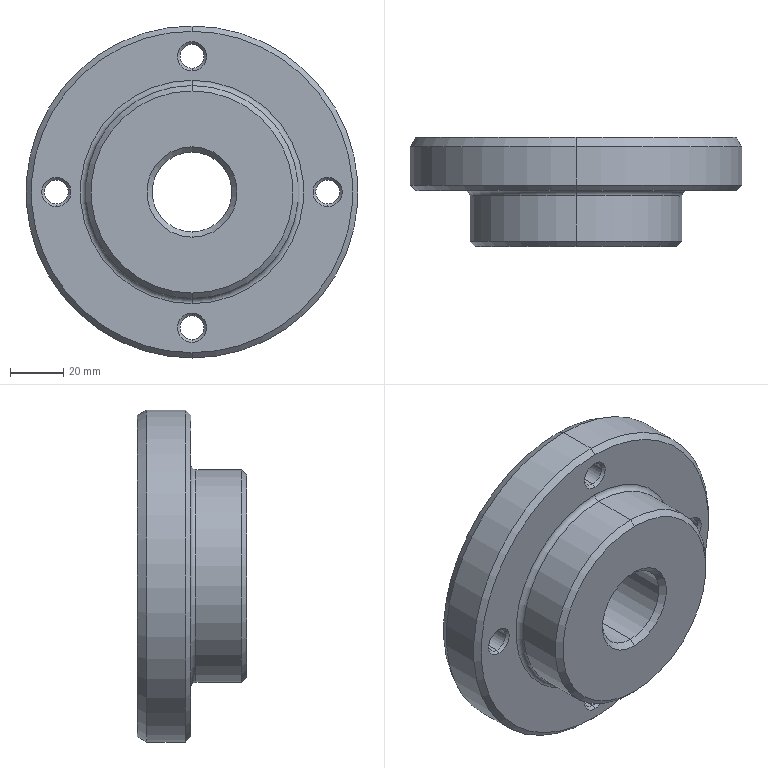Part | STEP file | Anel centralizador - Torre 1 cav | 1 solid | 57 faces | box 124.8 x 41 x 124.8 mm | volume 308667 mm3 | cone 26 | cylinder 22 | plane 7 | torus 2 | commonest cylinder face diameters 9 x8 15 x8 30 x2 80 x2 124.8 x2